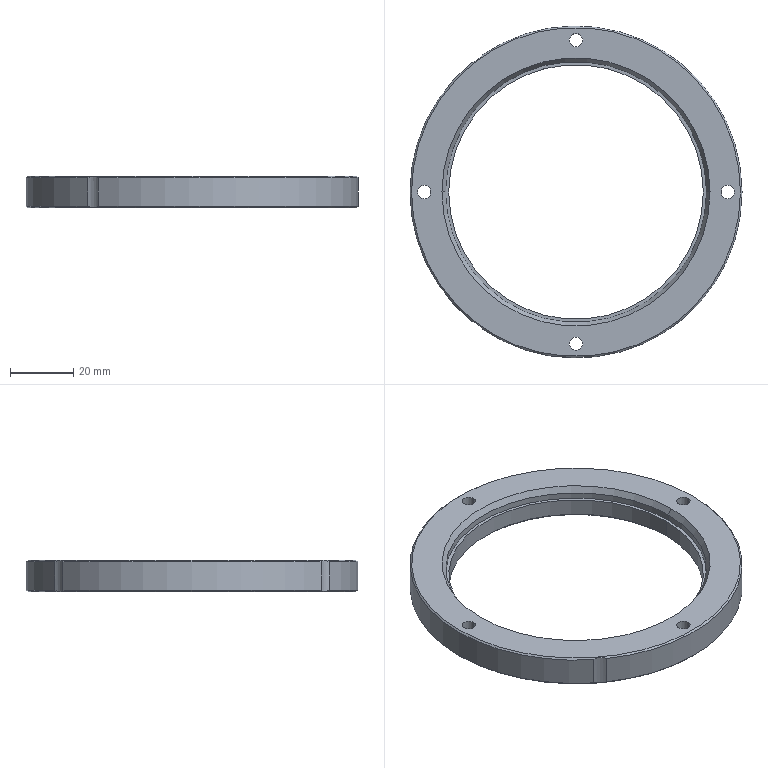Part | STEP file | 227H056250 JIG_Default | 1 solid | 28 faces | box 105 x 105 x 10 mm | volume 33679 mm3 | cylinder 17 | cone 8 | plane 3 | commonest cylinder face diameters 4.2 x8 105 x3 13 x2 80.5 x2 82.5 x2